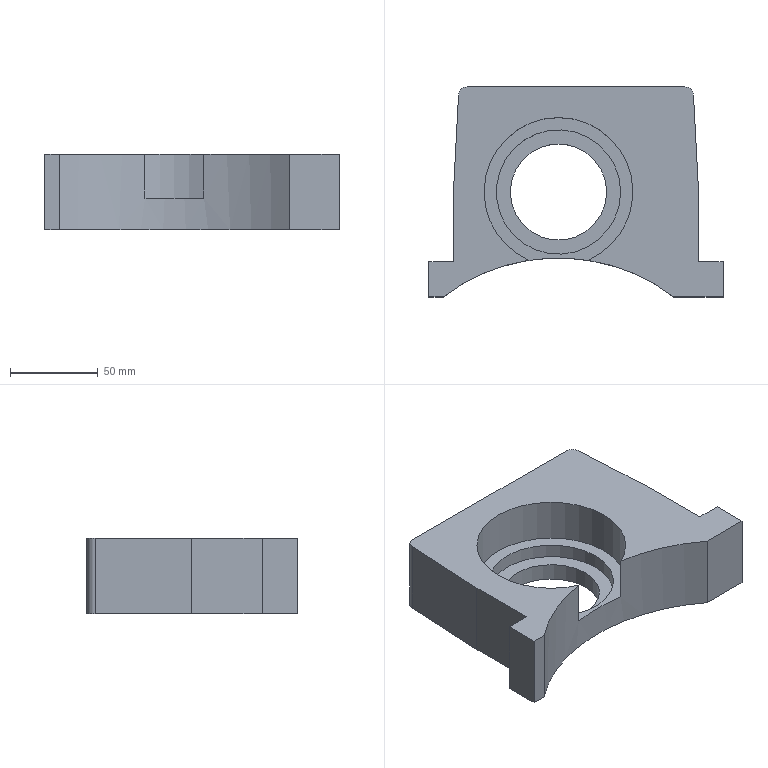Part | STEP file | SLIDE2-2_id594_x_t | 1 solid | 21 faces | box 168 x 120 x 43 mm | volume 457248 mm3 | plane 15 | cylinder 6 | commonest cylinder face diameters 10 x2 55 x1 71 x1 85 x1 217 x1
STEP:
#1=CARTESIAN_POINT('',(5.5,0.,82.003));
#2=VERTEX_POINT('',#1);
#3=CARTESIAN_POINT('',(-30.,0.,82.003));
#4=DIRECTION('',(0.,0.,1.));
#5=DIRECTION('',(1.,0.,0.));
#6=AXIS2_PLACEMENT_3D('',#3,#4,#5);
#7=CIRCLE('',#6,35.5);
#8=EDGE_CURVE('',#2,#2,#7,.T.);
#9=ORIENTED_EDGE('',*,*,#8,.F.);
#10=EDGE_LOOP('',(#9));
#11=FACE_BOUND('',#10,.T.);
#12=CARTESIAN_POINT('',(5.5,0.,90.003));
#13=VERTEX_POINT('',#12);
#14=CARTESIAN_POINT('',(-30.,0.,90.003));
#15=DIRECTION('',(0.,0.,-1.));
#16=DIRECTION('',(1.,0.,0.));
#17=AXIS2_PLACEMENT_3D('',#14,#15,#16);
#18=CIRCLE('',#17,35.5);
#19=EDGE_CURVE('',#13,#13,#18,.T.);
#20=ORIENTED_EDGE('',*,*,#19,.F.);
#21=EDGE_LOOP('',(#20));
#22=FACE_BOUND('',#21,.T.);
#23=CARTESIAN_POINT('',(-30.,0.,115.003));
#24=DIRECTION('',(0.,0.,1.));
#25=DIRECTION('',(1.,0.,0.));
#26=AXIS2_PLACEMENT_3D('',#23,#24,#25);
#27=CYLINDRICAL_SURFACE('',#26,35.5);
#28=ADVANCED_FACE('',(#11,#22),#27,.F.);
#29=ORIENTED_EDGE('',*,*,#19,.T.);
#30=EDGE_LOOP('',(#29));
#31=FACE_BOUND('',#30,.T.);
#32=CARTESIAN_POINT('',(-13.149,-39.017,90.003));
#33=VERTEX_POINT('',#32);
#34=CARTESIAN_POINT('',(-46.851,-39.017,90.003));
#35=VERTEX_POINT('',#34);
#36=CARTESIAN_POINT('',(-30.,0.,90.003));
#37=DIRECTION('',(0.,0.,1.));
#38=DIRECTION('',(1.,0.,0.));
#39=AXIS2_PLACEMENT_3D('',#36,#37,#38);
#40=CIRCLE('',#39,42.5);
#41=EDGE_CURVE('',#33,#35,#40,.T.);
#42=ORIENTED_EDGE('',*,*,#41,.T.);
#43=CARTESIAN_POINT('',(-30.,-146.2,90.003));
#44=DIRECTION('',(0.,0.,-1.));
#45=DIRECTION('',(1.,0.,0.));
#46=AXIS2_PLACEMENT_3D('',#43,#44,#45);
#47=CIRCLE('',#46,108.5);
#48=EDGE_CURVE('',#35,#33,#47,.T.);
#49=ORIENTED_EDGE('',*,*,#48,.T.);
#50=EDGE_LOOP('',(#42,#49));
#51=FACE_BOUND('',#50,.T.);
#52=CARTESIAN_POINT('',(50.,60.,90.003));
#53=DIRECTION('',(0.,0.,1.));
#54=DIRECTION('',(1.,0.,0.));
#55=AXIS2_PLACEMENT_3D('',#52,#53,#54);
#56=PLANE('',#55);
#57=ADVANCED_FACE('',(#31,#51),#56,.T.);
#58=ORIENTED_EDGE('',*,*,#41,.F.);
#59=CARTESIAN_POINT('',(-13.149,-39.017,115.003));
#60=VERTEX_POINT('',#59);
#61=CARTESIAN_POINT('',(-13.149,-39.017,145.5));
#62=DIRECTION('',(0.,0.,1.));
#63=VECTOR('',#62,1.);
#64=LINE('',#61,#63);
#65=EDGE_CURVE('',#33,#60,#64,.T.);
#66=ORIENTED_EDGE('',*,*,#65,.T.);
#67=CARTESIAN_POINT('',(-46.851,-39.017,115.003));
#68=VERTEX_POINT('',#67);
#69=CARTESIAN_POINT('',(-30.,0.,115.003));
#70=DIRECTION('',(0.,0.,-1.));
#71=DIRECTION('',(1.,0.,0.));
#72=AXIS2_PLACEMENT_3D('',#69,#70,#71);
#73=CIRCLE('',#72,42.5);
#74=EDGE_CURVE('',#68,#60,#73,.T.);
#75=ORIENTED_EDGE('',*,*,#74,.F.);
#76=CARTESIAN_POINT('',(-46.851,-39.017,145.5));
#77=DIRECTION('',(0.,0.,-1.));
#78=VECTOR('',#77,1.);
#79=LINE('',#76,#78);
#80=EDGE_CURVE('',#68,#35,#79,.T.);
#81=ORIENTED_EDGE('',*,*,#80,.T.);
#82=EDGE_LOOP('',(#58,#66,#75,#81));
#83=FACE_OUTER_BOUND('',#82,.T.);
#84=CARTESIAN_POINT('',(-30.,0.,115.003));
#85=DIRECTION('',(0.,0.,1.));
#86=DIRECTION('',(1.,0.,0.));
#87=AXIS2_PLACEMENT_3D('',#84,#85,#86);
#88=CYLINDRICAL_SURFACE('',#87,42.5);
#89=ADVANCED_FACE('',(#83),#88,.F.);
#90=CARTESIAN_POINT('',(50.,0.05468,115.003));
#91=VERTEX_POINT('',#90);
#92=CARTESIAN_POINT('',(50.,-40.,115.003));
#93=VERTEX_POINT('',#92);
#94=CARTESIAN_POINT('',(50.,-50.,115.003));
#95=DIRECTION('',(0.,-1.,0.));
#96=VECTOR('',#95,1.);
#97=LINE('',#94,#96);
#98=EDGE_CURVE('',#91,#93,#97,.T.);
#99=ORIENTED_EDGE('',*,*,#98,.F.);
#100=CARTESIAN_POINT('',(47.107,55.262,115.003));
#101=VERTEX_POINT('',#100);
#102=CARTESIAN_POINT('',(50.,0.05468,115.003));
#103=DIRECTION('',(-0.05234,0.9986,0.));
#104=VECTOR('',#103,1.);
#105=LINE('',#102,#104);
#106=EDGE_CURVE('',#91,#101,#105,.T.);
#107=ORIENTED_EDGE('',*,*,#106,.T.);
#108=CARTESIAN_POINT('',(42.114,60.,115.003));
#109=VERTEX_POINT('',#108);
#110=CARTESIAN_POINT('',(42.114,55.,115.003));
#111=DIRECTION('',(0.,0.,-1.));
#112=DIRECTION('',(-1.,0.,0.));
#113=AXIS2_PLACEMENT_3D('',#110,#111,#112);
#114=CIRCLE('',#113,5.);
#115=EDGE_CURVE('',#109,#101,#114,.T.);
#116=ORIENTED_EDGE('',*,*,#115,.F.);
#117=CARTESIAN_POINT('',(-82.114,60.,115.003));
#118=VERTEX_POINT('',#117);
#119=CARTESIAN_POINT('',(50.,60.,115.003));
#120=DIRECTION('',(1.,0.,0.));
#121=VECTOR('',#120,1.);
#122=LINE('',#119,#121);
#123=EDGE_CURVE('',#118,#109,#122,.T.);
#124=ORIENTED_EDGE('',*,*,#123,.F.);
#125=CARTESIAN_POINT('',(-87.107,55.262,115.003));
#126=VERTEX_POINT('',#125);
#127=CARTESIAN_POINT('',(-82.114,55.,115.003));
#128=DIRECTION('',(0.,0.,-1.));
#129=DIRECTION('',(-1.,0.,0.));
#130=AXIS2_PLACEMENT_3D('',#127,#128,#129);
#131=CIRCLE('',#130,5.);
#132=EDGE_CURVE('',#126,#118,#131,.T.);
#133=ORIENTED_EDGE('',*,*,#132,.F.);
#134=CARTESIAN_POINT('',(-90.,0.05468,115.003));
#135=VERTEX_POINT('',#134);
#136=CARTESIAN_POINT('',(-87.107,55.262,115.003));
#137=DIRECTION('',(-0.05234,-0.9986,0.));
#138=VECTOR('',#137,1.);
#139=LINE('',#136,#138);
#140=EDGE_CURVE('',#126,#135,#139,.T.);
#141=ORIENTED_EDGE('',*,*,#140,.T.);
#142=CARTESIAN_POINT('',(-90.,-40.,115.003));
#143=VERTEX_POINT('',#142);
#144=CARTESIAN_POINT('',(-90.,60.,115.003));
#145=DIRECTION('',(0.,1.,0.));
#146=VECTOR('',#145,1.);
#147=LINE('',#144,#146);
#148=EDGE_CURVE('',#143,#135,#147,.T.);
#149=ORIENTED_EDGE('',*,*,#148,.F.);
#150=CARTESIAN_POINT('',(-104.,-40.,115.003));
#151=VERTEX_POINT('',#150);
#152=CARTESIAN_POINT('',(-90.,-40.,115.003));
#153=DIRECTION('',(1.,0.,0.));
#154=VECTOR('',#153,1.);
#155=LINE('',#152,#154);
#156=EDGE_CURVE('',#151,#143,#155,.T.);
#157=ORIENTED_EDGE('',*,*,#156,.F.);
#158=CARTESIAN_POINT('',(-104.,-60.,115.003));
#159=VERTEX_POINT('',#158);
#160=CARTESIAN_POINT('',(-104.,-50.,115.003));
#161=DIRECTION('',(0.,1.,0.));
#162=VECTOR('',#161,1.);
#163=LINE('',#160,#162);
#164=EDGE_CURVE('',#159,#151,#163,.T.);
#165=ORIENTED_EDGE('',*,*,#164,.F.);
#166=CARTESIAN_POINT('',(-95.892,-60.,115.003));
#167=VERTEX_POINT('',#166);
#168=CARTESIAN_POINT('',(-98.,-60.,115.003));
#169=DIRECTION('',(-1.,0.,0.));
#170=VECTOR('',#169,1.);
#171=LINE('',#168,#170);
#172=EDGE_CURVE('',#167,#159,#171,.T.);
#173=ORIENTED_EDGE('',*,*,#172,.F.);
#174=CARTESIAN_POINT('',(-30.,-146.2,115.003));
#175=DIRECTION('',(0.,0.,-1.));
#176=DIRECTION('',(1.,0.,0.));
#177=AXIS2_PLACEMENT_3D('',#174,#175,#176);
#178=CIRCLE('',#177,108.5);
#179=EDGE_CURVE('',#167,#68,#178,.T.);
#180=ORIENTED_EDGE('',*,*,#179,.T.);
#181=ORIENTED_EDGE('',*,*,#74,.T.);
#182=CARTESIAN_POINT('',(35.892,-60.,115.003));
#183=VERTEX_POINT('',#182);
#184=CARTESIAN_POINT('',(-30.,-146.2,115.003));
#185=DIRECTION('',(0.,0.,-1.));
#186=DIRECTION('',(1.,0.,0.));
#187=AXIS2_PLACEMENT_3D('',#184,#185,#186);
#188=CIRCLE('',#187,108.5);
#189=EDGE_CURVE('',#60,#183,#188,.T.);
#190=ORIENTED_EDGE('',*,*,#189,.T.);
#191=CARTESIAN_POINT('',(64.,-60.,115.003));
#192=VERTEX_POINT('',#191);
#193=CARTESIAN_POINT('',(-98.,-60.,115.003));
#194=DIRECTION('',(-1.,0.,0.));
#195=VECTOR('',#194,1.);
#196=LINE('',#193,#195);
#197=EDGE_CURVE('',#192,#183,#196,.T.);
#198=ORIENTED_EDGE('',*,*,#197,.F.);
#199=CARTESIAN_POINT('',(64.,-40.,115.003));
#200=VERTEX_POINT('',#199);
#201=CARTESIAN_POINT('',(64.,-60.,115.003));
#202=DIRECTION('',(0.,-1.,0.));
#203=VECTOR('',#202,1.);
#204=LINE('',#201,#203);
#205=EDGE_CURVE('',#200,#192,#204,.T.);
#206=ORIENTED_EDGE('',*,*,#205,.F.);
#207=CARTESIAN_POINT('',(58.,-40.,115.003));
#208=DIRECTION('',(1.,0.,0.));
#209=VECTOR('',#208,1.);
#210=LINE('',#207,#209);
#211=EDGE_CURVE('',#93,#200,#210,.T.);
#212=ORIENTED_EDGE('',*,*,#211,.F.);
#213=EDGE_LOOP('',(#99,#107,#116,#124,#133,#141,#149,#157,#165,#173,#180,#181,#190,#198,#206,#212));
#214=FACE_OUTER_BOUND('',#213,.T.);
#215=CARTESIAN_POINT('',(50.,60.,115.003));
#216=DIRECTION('',(0.,0.,1.));
#217=DIRECTION('',(1.,0.,0.));
#218=AXIS2_PLACEMENT_3D('',#215,#216,#217);
#219=PLANE('',#218);
#220=ADVANCED_FACE('',(#214),#219,.T.);
#221=CARTESIAN_POINT('',(-2.5,0.,82.003));
#222=VERTEX_POINT('',#221);
#223=CARTESIAN_POINT('',(-30.,0.,82.003));
#224=DIRECTION('',(0.,0.,-1.));
#225=DIRECTION('',(1.,0.,0.));
#226=AXIS2_PLACEMENT_3D('',#223,#224,#225);
#227=CIRCLE('',#226,27.5);
#228=EDGE_CURVE('',#222,#222,#227,.T.);
#229=ORIENTED_EDGE('',*,*,#228,.T.);
#230=EDGE_LOOP('',(#229));
#231=FACE_BOUND('',#230,.T.);
#232=ORIENTED_EDGE('',*,*,#8,.T.);
#233=EDGE_LOOP('',(#232));
#234=FACE_BOUND('',#233,.T.);
#235=CARTESIAN_POINT('',(50.,60.,82.003));
#236=DIRECTION('',(0.,0.,1.));
#237=DIRECTION('',(1.,0.,0.));
#238=AXIS2_PLACEMENT_3D('',#235,#236,#237);
#239=PLANE('',#238);
#240=ADVANCED_FACE('',(#231,#234),#239,.T.);
#241=ORIENTED_EDGE('',*,*,#106,.F.);
#242=CARTESIAN_POINT('',(50.,0.05468,72.003));
#243=VERTEX_POINT('',#242);
#244=CARTESIAN_POINT('',(50.,0.05468,72.003));
#245=DIRECTION('',(0.,0.,1.));
#246=VECTOR('',#245,1.);
#247=LINE('',#244,#246);
#248=EDGE_CURVE('',#243,#91,#247,.T.);
#249=ORIENTED_EDGE('',*,*,#248,.F.);
#250=CARTESIAN_POINT('',(47.107,55.262,72.003));
#251=VERTEX_POINT('',#250);
#252=CARTESIAN_POINT('',(50.,0.05468,72.003));
#253=DIRECTION('',(-0.05234,0.9986,0.));
#254=VECTOR('',#253,1.);
#255=LINE('',#252,#254);
#256=EDGE_CURVE('',#243,#251,#255,.T.);
#257=ORIENTED_EDGE('',*,*,#256,.T.);
#258=CARTESIAN_POINT('',(47.107,55.262,72.003));
#259=DIRECTION('',(0.,0.,-1.));
#260=VECTOR('',#259,1.);
#261=LINE('',#258,#260);
#262=EDGE_CURVE('',#101,#251,#261,.T.);
#263=ORIENTED_EDGE('',*,*,#262,.F.);
#264=EDGE_LOOP('',(#241,#249,#257,#263));
#265=FACE_OUTER_BOUND('',#264,.T.);
#266=CARTESIAN_POINT('',(50.,0.05468,72.003));
#267=DIRECTION('',(-0.9986,-0.05234,0.));
#268=DIRECTION('',(0.05234,-0.9986,0.));
#269=AXIS2_PLACEMENT_3D('',#266,#267,#268);
#270=PLANE('',#269);
#271=ADVANCED_FACE('',(#265),#270,.F.);
#272=ORIENTED_EDGE('',*,*,#262,.T.);
#273=CARTESIAN_POINT('',(42.114,60.,72.003));
#274=VERTEX_POINT('',#273);
#275=CARTESIAN_POINT('',(42.114,55.,72.003));
#276=DIRECTION('',(0.,0.,1.));
#277=DIRECTION('',(-1.,0.,0.));
#278=AXIS2_PLACEMENT_3D('',#275,#276,#277);
#279=CIRCLE('',#278,5.);
#280=EDGE_CURVE('',#251,#274,#279,.T.);
#281=ORIENTED_EDGE('',*,*,#280,.T.);
#282=CARTESIAN_POINT('',(42.114,60.,72.003));
#283=DIRECTION('',(0.,0.,-1.));
#284=VECTOR('',#283,1.);
#285=LINE('',#282,#284);
#286=EDGE_CURVE('',#109,#274,#285,.T.);
#287=ORIENTED_EDGE('',*,*,#286,.F.);
#288=ORIENTED_EDGE('',*,*,#115,.T.);
#289=EDGE_LOOP('',(#272,#281,#287,#288));
#290=FACE_OUTER_BOUND('',#289,.T.);
#291=CARTESIAN_POINT('',(42.114,55.,72.003));
#292=DIRECTION('',(0.,0.,-1.));
#293=DIRECTION('',(-1.,0.,0.));
#294=AXIS2_PLACEMENT_3D('',#291,#292,#293);
#295=CYLINDRICAL_SURFACE('',#294,5.);
#296=ADVANCED_FACE('',(#290),#295,.T.);
#297=ORIENTED_EDGE('',*,*,#123,.T.);
#298=ORIENTED_EDGE('',*,*,#286,.T.);
#299=CARTESIAN_POINT('',(-82.114,60.,72.003));
#300=VERTEX_POINT('',#299);
#301=CARTESIAN_POINT('',(50.,60.,72.003));
#302=DIRECTION('',(-1.,0.,0.));
#303=VECTOR('',#302,1.);
#304=LINE('',#301,#303);
#305=EDGE_CURVE('',#274,#300,#304,.T.);
#306=ORIENTED_EDGE('',*,*,#305,.T.);
#307=CARTESIAN_POINT('',(-82.114,60.,72.003));
#308=DIRECTION('',(0.,0.,-1.));
#309=VECTOR('',#308,1.);
#310=LINE('',#307,#309);
#311=EDGE_CURVE('',#118,#300,#310,.T.);
#312=ORIENTED_EDGE('',*,*,#311,.F.);
#313=EDGE_LOOP('',(#297,#298,#306,#312));
#314=FACE_OUTER_BOUND('',#313,.T.);
#315=CARTESIAN_POINT('',(50.,60.,72.003));
#316=DIRECTION('',(0.,1.,0.));
#317=DIRECTION('',(0.,0.,1.));
#318=AXIS2_PLACEMENT_3D('',#315,#316,#317);
#319=PLANE('',#318);
#320=ADVANCED_FACE('',(#314),#319,.T.);
#321=ORIENTED_EDGE('',*,*,#311,.T.);
#322=CARTESIAN_POINT('',(-87.107,55.262,72.003));
#323=VERTEX_POINT('',#322);
#324=CARTESIAN_POINT('',(-82.114,55.,72.003));
#325=DIRECTION('',(0.,0.,1.));
#326=DIRECTION('',(-1.,0.,0.));
#327=AXIS2_PLACEMENT_3D('',#324,#325,#326);
#328=CIRCLE('',#327,5.);
#329=EDGE_CURVE('',#300,#323,#328,.T.);
#330=ORIENTED_EDGE('',*,*,#329,.T.);
#331=CARTESIAN_POINT('',(-87.107,55.262,72.003));
#332=DIRECTION('',(0.,0.,1.));
#333=VECTOR('',#332,1.);
#334=LINE('',#331,#333);
#335=EDGE_CURVE('',#323,#126,#334,.T.);
#336=ORIENTED_EDGE('',*,*,#335,.T.);
#337=ORIENTED_EDGE('',*,*,#132,.T.);
#338=EDGE_LOOP('',(#321,#330,#336,#337));
#339=FACE_OUTER_BOUND('',#338,.T.);
#340=CARTESIAN_POINT('',(-82.114,55.,72.003));
#341=DIRECTION('',(0.,0.,-1.));
#342=DIRECTION('',(-1.,0.,0.));
#343=AXIS2_PLACEMENT_3D('',#340,#341,#342);
#344=CYLINDRICAL_SURFACE('',#343,5.);
#345=ADVANCED_FACE('',(#339),#344,.T.);
#346=ORIENTED_EDGE('',*,*,#140,.F.);
#347=ORIENTED_EDGE('',*,*,#335,.F.);
#348=CARTESIAN_POINT('',(-90.,0.05468,72.003));
#349=VERTEX_POINT('',#348);
#350=CARTESIAN_POINT('',(-87.107,55.262,72.003));
#351=DIRECTION('',(-0.05234,-0.9986,0.));
#352=VECTOR('',#351,1.);
#353=LINE('',#350,#352);
#354=EDGE_CURVE('',#323,#349,#353,.T.);
#355=ORIENTED_EDGE('',*,*,#354,.T.);
#356=CARTESIAN_POINT('',(-90.,0.05468,72.003));
#357=DIRECTION('',(0.,0.,-1.));
#358=VECTOR('',#357,1.);
#359=LINE('',#356,#358);
#360=EDGE_CURVE('',#135,#349,#359,.T.);
#361=ORIENTED_EDGE('',*,*,#360,.F.);
#362=EDGE_LOOP('',(#346,#347,#355,#361));
#363=FACE_OUTER_BOUND('',#362,.T.);
#364=CARTESIAN_POINT('',(-87.107,55.262,72.003));
#365=DIRECTION('',(0.9986,-0.05234,0.));
#366=DIRECTION('',(0.05234,0.9986,0.));
#367=AXIS2_PLACEMENT_3D('',#364,#365,#366);
#368=PLANE('',#367);
#369=ADVANCED_FACE('',(#363),#368,.F.);
#370=ORIENTED_EDGE('',*,*,#148,.T.);
#371=ORIENTED_EDGE('',*,*,#360,.T.);
#372=CARTESIAN_POINT('',(-90.,-40.,72.003));
#373=VERTEX_POINT('',#372);
#374=CARTESIAN_POINT('',(-90.,60.,72.003));
#375=DIRECTION('',(0.,-1.,0.));
#376=VECTOR('',#375,1.);
#377=LINE('',#374,#376);
#378=EDGE_CURVE('',#349,#373,#377,.T.);
#379=ORIENTED_EDGE('',*,*,#378,.T.);
#380=CARTESIAN_POINT('',(-90.,-40.,72.003));
#381=DIRECTION('',(0.,0.,-1.));
#382=VECTOR('',#381,1.);
#383=LINE('',#380,#382);
#384=EDGE_CURVE('',#143,#373,#383,.T.);
#385=ORIENTED_EDGE('',*,*,#384,.F.);
#386=EDGE_LOOP('',(#370,#371,#379,#385));
#387=FACE_OUTER_BOUND('',#386,.T.);
#388=CARTESIAN_POINT('',(-90.,60.,72.003));
#389=DIRECTION('',(-1.,0.,0.));
#390=DIRECTION('',(0.,0.,1.));
#391=AXIS2_PLACEMENT_3D('',#388,#389,#390);
#392=PLANE('',#391);
#393=ADVANCED_FACE('',(#387),#392,.T.);
#394=ORIENTED_EDGE('',*,*,#384,.T.);
#395=CARTESIAN_POINT('',(-104.,-40.,72.003));
#396=VERTEX_POINT('',#395);
#397=CARTESIAN_POINT('',(50.,-40.,72.003));
#398=DIRECTION('',(-1.,0.,0.));
#399=VECTOR('',#398,1.);
#400=LINE('',#397,#399);
#401=EDGE_CURVE('',#373,#396,#400,.T.);
#402=ORIENTED_EDGE('',*,*,#401,.T.);
#403=CARTESIAN_POINT('',(-104.,-40.,72.003));
#404=DIRECTION('',(0.,0.,-1.));
#405=VECTOR('',#404,1.);
#406=LINE('',#403,#405);
#407=EDGE_CURVE('',#151,#396,#406,.T.);
#408=ORIENTED_EDGE('',*,*,#407,.F.);
#409=ORIENTED_EDGE('',*,*,#156,.T.);
#410=EDGE_LOOP('',(#394,#402,#408,#409));
#411=FACE_OUTER_BOUND('',#410,.T.);
#412=CARTESIAN_POINT('',(-90.,-40.,72.003));
#413=DIRECTION('',(0.,1.,0.));
#414=DIRECTION('',(0.,0.,1.));
#415=AXIS2_PLACEMENT_3D('',#412,#413,#414);
#416=PLANE('',#415);
#417=ADVANCED_FACE('',(#411),#416,.T.);
#418=ORIENTED_EDGE('',*,*,#407,.T.);
#419=CARTESIAN_POINT('',(-104.,-60.,72.003));
#420=VERTEX_POINT('',#419);
#421=CARTESIAN_POINT('',(-104.,60.,72.003));
#422=DIRECTION('',(0.,-1.,0.));
#423=VECTOR('',#422,1.);
#424=LINE('',#421,#423);
#425=EDGE_CURVE('',#396,#420,#424,.T.);
#426=ORIENTED_EDGE('',*,*,#425,.T.);
#427=CARTESIAN_POINT('',(-104.,-60.,72.003));
#428=DIRECTION('',(0.,0.,-1.));
#429=VECTOR('',#428,1.);
#430=LINE('',#427,#429);
#431=EDGE_CURVE('',#159,#420,#430,.T.);
#432=ORIENTED_EDGE('',*,*,#431,.F.);
#433=ORIENTED_EDGE('',*,*,#164,.T.);
#434=EDGE_LOOP('',(#418,#426,#432,#433));
#435=FACE_OUTER_BOUND('',#434,.T.);
#436=CARTESIAN_POINT('',(-104.,-50.,72.003));
#437=DIRECTION('',(-1.,0.,0.));
#438=DIRECTION('',(0.,0.,1.));
#439=AXIS2_PLACEMENT_3D('',#436,#437,#438);
#440=PLANE('',#439);
#441=ADVANCED_FACE('',(#435),#440,.T.);
#442=CARTESIAN_POINT('',(-95.892,-60.,72.003));
#443=VERTEX_POINT('',#442);
#444=CARTESIAN_POINT('',(50.,-60.,72.003));
#445=DIRECTION('',(1.,0.,0.));
#446=VECTOR('',#445,1.);
#447=LINE('',#444,#446);
#448=EDGE_CURVE('',#420,#443,#447,.T.);
#449=ORIENTED_EDGE('',*,*,#448,.T.);
#450=CARTESIAN_POINT('',(-95.892,-60.,145.5));
#451=DIRECTION('',(0.,0.,1.));
#452=VECTOR('',#451,1.);
#453=LINE('',#450,#452);
#454=EDGE_CURVE('',#443,#167,#453,.T.);
#455=ORIENTED_EDGE('',*,*,#454,.T.);
#456=ORIENTED_EDGE('',*,*,#172,.T.);
#457=ORIENTED_EDGE('',*,*,#431,.T.);
#458=EDGE_LOOP('',(#449,#455,#456,#457));
#459=FACE_OUTER_BOUND('',#458,.T.);
#460=CARTESIAN_POINT('',(-98.,-60.,72.003));
#461=DIRECTION('',(0.,-1.,0.));
#462=DIRECTION('',(0.,0.,-1.));
#463=AXIS2_PLACEMENT_3D('',#460,#461,#462);
#464=PLANE('',#463);
#465=ADVANCED_FACE('',(#459),#464,.T.);
#466=ORIENTED_EDGE('',*,*,#189,.F.);
#467=ORIENTED_EDGE('',*,*,#65,.F.);
#468=ORIENTED_EDGE('',*,*,#48,.F.);
#469=ORIENTED_EDGE('',*,*,#80,.F.);
#470=ORIENTED_EDGE('',*,*,#179,.F.);
#471=ORIENTED_EDGE('',*,*,#454,.F.);
#472=CARTESIAN_POINT('',(35.892,-60.,72.003));
#473=VERTEX_POINT('',#472);
#474=CARTESIAN_POINT('',(-30.,-146.2,72.003));
#475=DIRECTION('',(0.,0.,-1.));
#476=DIRECTION('',(1.,0.,0.));
#477=AXIS2_PLACEMENT_3D('',#474,#475,#476);
#478=CIRCLE('',#477,108.5);
#479=EDGE_CURVE('',#443,#473,#478,.T.);
#480=ORIENTED_EDGE('',*,*,#479,.T.);
#481=CARTESIAN_POINT('',(35.892,-60.,72.003));
#482=DIRECTION('',(0.,0.,-1.));
#483=VECTOR('',#482,1.);
#484=LINE('',#481,#483);
#485=EDGE_CURVE('',#183,#473,#484,.T.);
#486=ORIENTED_EDGE('',*,*,#485,.F.);
#487=EDGE_LOOP('',(#466,#467,#468,#469,#470,#471,#480,#486));
#488=FACE_OUTER_BOUND('',#487,.T.);
#489=CARTESIAN_POINT('',(-30.,-146.2,145.5));
#490=DIRECTION('',(0.,0.,1.));
#491=DIRECTION('',(1.,0.,0.));
#492=AXIS2_PLACEMENT_3D('',#489,#490,#491);
#493=CYLINDRICAL_SURFACE('',#492,108.5);
#494=ADVANCED_FACE('',(#488),#493,.F.);
#495=ORIENTED_EDGE('',*,*,#197,.T.);
#496=ORIENTED_EDGE('',*,*,#485,.T.);
#497=CARTESIAN_POINT('',(64.,-60.,72.003));
#498=VERTEX_POINT('',#497);
#499=CARTESIAN_POINT('',(50.,-60.,72.003));
#500=DIRECTION('',(1.,0.,0.));
#501=VECTOR('',#500,1.);
#502=LINE('',#499,#501);
#503=EDGE_CURVE('',#473,#498,#502,.T.);
#504=ORIENTED_EDGE('',*,*,#503,.T.);
#505=CARTESIAN_POINT('',(64.,-60.,72.003));
#506=DIRECTION('',(0.,0.,-1.));
#507=VECTOR('',#506,1.);
#508=LINE('',#505,#507);
#509=EDGE_CURVE('',#192,#498,#508,.T.);
#510=ORIENTED_EDGE('',*,*,#509,.F.);
#511=EDGE_LOOP('',(#495,#496,#504,#510));
#512=FACE_OUTER_BOUND('',#511,.T.);
#513=CARTESIAN_POINT('',(-98.,-60.,72.003));
#514=DIRECTION('',(0.,-1.,0.));
#515=DIRECTION('',(0.,0.,-1.));
#516=AXIS2_PLACEMENT_3D('',#513,#514,#515);
#517=PLANE('',#516);
#518=ADVANCED_FACE('',(#512),#517,.T.);
#519=ORIENTED_EDGE('',*,*,#509,.T.);
#520=CARTESIAN_POINT('',(64.,-40.,72.003));
#521=VERTEX_POINT('',#520);
#522=CARTESIAN_POINT('',(64.,60.,72.003));
#523=DIRECTION('',(0.,1.,0.));
#524=VECTOR('',#523,1.);
#525=LINE('',#522,#524);
#526=EDGE_CURVE('',#498,#521,#525,.T.);
#527=ORIENTED_EDGE('',*,*,#526,.T.);
#528=CARTESIAN_POINT('',(64.,-40.,72.003));
#529=DIRECTION('',(0.,0.,-1.));
#530=VECTOR('',#529,1.);
#531=LINE('',#528,#530);
#532=EDGE_CURVE('',#200,#521,#531,.T.);
#533=ORIENTED_EDGE('',*,*,#532,.F.);
#534=ORIENTED_EDGE('',*,*,#205,.T.);
#535=EDGE_LOOP('',(#519,#527,#533,#534));
#536=FACE_OUTER_BOUND('',#535,.T.);
#537=CARTESIAN_POINT('',(64.,-60.,72.003));
#538=DIRECTION('',(1.,0.,0.));
#539=DIRECTION('',(0.,0.,-1.));
#540=AXIS2_PLACEMENT_3D('',#537,#538,#539);
#541=PLANE('',#540);
#542=ADVANCED_FACE('',(#536),#541,.T.);
#543=ORIENTED_EDGE('',*,*,#532,.T.);
#544=CARTESIAN_POINT('',(50.,-40.,72.003));
#545=VERTEX_POINT('',#544);
#546=CARTESIAN_POINT('',(50.,-40.,72.003));
#547=DIRECTION('',(-1.,0.,0.));
#548=VECTOR('',#547,1.);
#549=LINE('',#546,#548);
#550=EDGE_CURVE('',#521,#545,#549,.T.);
#551=ORIENTED_EDGE('',*,*,#550,.T.);
#552=CARTESIAN_POINT('',(50.,-40.,72.003));
#553=DIRECTION('',(0.,0.,-1.));
#554=VECTOR('',#553,1.);
#555=LINE('',#552,#554);
#556=EDGE_CURVE('',#93,#545,#555,.T.);
#557=ORIENTED_EDGE('',*,*,#556,.F.);
#558=ORIENTED_EDGE('',*,*,#211,.T.);
#559=EDGE_LOOP('',(#543,#551,#557,#558));
#560=FACE_OUTER_BOUND('',#559,.T.);
#561=CARTESIAN_POINT('',(58.,-40.,72.003));
#562=DIRECTION('',(0.,1.,0.));
#563=DIRECTION('',(0.,0.,1.));
#564=AXIS2_PLACEMENT_3D('',#561,#562,#563);
#565=PLANE('',#564);
#566=ADVANCED_FACE('',(#560),#565,.T.);
#567=CARTESIAN_POINT('',(50.,60.,72.003));
#568=DIRECTION('',(0.,1.,0.));
#569=VECTOR('',#568,1.);
#570=LINE('',#567,#569);
#571=EDGE_CURVE('',#545,#243,#570,.T.);
#572=ORIENTED_EDGE('',*,*,#571,.T.);
#573=ORIENTED_EDGE('',*,*,#248,.T.);
#574=ORIENTED_EDGE('',*,*,#98,.T.);
#575=ORIENTED_EDGE('',*,*,#556,.T.);
#576=EDGE_LOOP('',(#572,#573,#574,#575));
#577=FACE_OUTER_BOUND('',#576,.T.);
#578=CARTESIAN_POINT('',(50.,-50.,72.003));
#579=DIRECTION('',(1.,0.,0.));
#580=DIRECTION('',(0.,0.,-1.));
#581=AXIS2_PLACEMENT_3D('',#578,#579,#580);
#582=PLANE('',#581);
#583=ADVANCED_FACE('',(#577),#582,.T.);
#584=CARTESIAN_POINT('',(-2.5,0.,72.003));
#585=VERTEX_POINT('',#584);
#586=CARTESIAN_POINT('',(-30.,0.,72.003));
#587=DIRECTION('',(0.,0.,-1.));
#588=DIRECTION('',(1.,0.,0.));
#589=AXIS2_PLACEMENT_3D('',#586,#587,#588);
#590=CIRCLE('',#589,27.5);
#591=EDGE_CURVE('',#585,#585,#590,.T.);
#592=ORIENTED_EDGE('',*,*,#591,.T.);
#593=EDGE_LOOP('',(#592));
#594=FACE_BOUND('',#593,.T.);
#595=ORIENTED_EDGE('',*,*,#228,.F.);
#596=EDGE_LOOP('',(#595));
#597=FACE_BOUND('',#596,.T.);
#598=CARTESIAN_POINT('',(-30.,0.,72.003));
#599=DIRECTION('',(0.,0.,1.));
#600=DIRECTION('',(1.,0.,0.));
#601=AXIS2_PLACEMENT_3D('',#598,#599,#600);
#602=CYLINDRICAL_SURFACE('',#601,27.5);
#603=ADVANCED_FACE('',(#594,#597),#602,.F.);
#604=ORIENTED_EDGE('',*,*,#591,.F.);
#605=EDGE_LOOP('',(#604));
#606=FACE_BOUND('',#605,.T.);
#607=ORIENTED_EDGE('',*,*,#550,.F.);
#608=ORIENTED_EDGE('',*,*,#526,.F.);
#609=ORIENTED_EDGE('',*,*,#503,.F.);
#610=ORIENTED_EDGE('',*,*,#479,.F.);
#611=ORIENTED_EDGE('',*,*,#448,.F.);
#612=ORIENTED_EDGE('',*,*,#425,.F.);
#613=ORIENTED_EDGE('',*,*,#401,.F.);
#614=ORIENTED_EDGE('',*,*,#378,.F.);
#615=ORIENTED_EDGE('',*,*,#354,.F.);
#616=ORIENTED_EDGE('',*,*,#329,.F.);
#617=ORIENTED_EDGE('',*,*,#305,.F.);
#618=ORIENTED_EDGE('',*,*,#280,.F.);
#619=ORIENTED_EDGE('',*,*,#256,.F.);
#620=ORIENTED_EDGE('',*,*,#571,.F.);
#621=EDGE_LOOP('',(#607,#608,#609,#610,#611,#612,#613,#614,#615,#616,#617,#618,#619,#620));
#622=FACE_BOUND('',#621,.T.);
#623=CARTESIAN_POINT('',(50.,60.,72.003));
#624=DIRECTION('',(0.,0.,1.));
#625=DIRECTION('',(1.,0.,0.));
#626=AXIS2_PLACEMENT_3D('',#623,#624,#625);
#627=PLANE('',#626);
#628=ADVANCED_FACE('',(#606,#622),#627,.F.);
#629=CLOSED_SHELL('',(#28,#57,#89,#220,#240,#271,#296,#320,#345,#369,#393,#417,#441,#465,#494,#518,#542,#566,#583,#603,#628));
#630=MANIFOLD_SOLID_BREP('',#629);
#631=(LENGTH_UNIT()NAMED_UNIT(*)SI_UNIT(.MILLI.,.METRE.));
#632=UNCERTAINTY_MEASURE_WITH_UNIT(LENGTH_MEASURE(0.00004123),#631,'','');
#633=(NAMED_UNIT(*)PLANE_ANGLE_UNIT()SI_UNIT($,.RADIAN.));
#634=PLANE_ANGLE_MEASURE_WITH_UNIT(PLANE_ANGLE_MEASURE(0.01745),#633);
#635=DIMENSIONAL_EXPONENTS(0.,0.,0.,0.,0.,0.,0.);
#636=(CONVERSION_BASED_UNIT('DEGREE',#634)NAMED_UNIT(#635)PLANE_ANGLE_UNIT());
#637=(NAMED_UNIT(*)SI_UNIT($,.STERADIAN.)SOLID_ANGLE_UNIT());
#638=(GEOMETRIC_REPRESENTATION_CONTEXT(3)GLOBAL_UNCERTAINTY_ASSIGNED_CONTEXT((#632))GLOBAL_UNIT_ASSIGNED_CONTEXT((#631,#636,#637))REPRESENTATION_CONTEXT('',''));
#639=ADVANCED_BREP_SHAPE_REPRESENTATION('',(#630),#638);